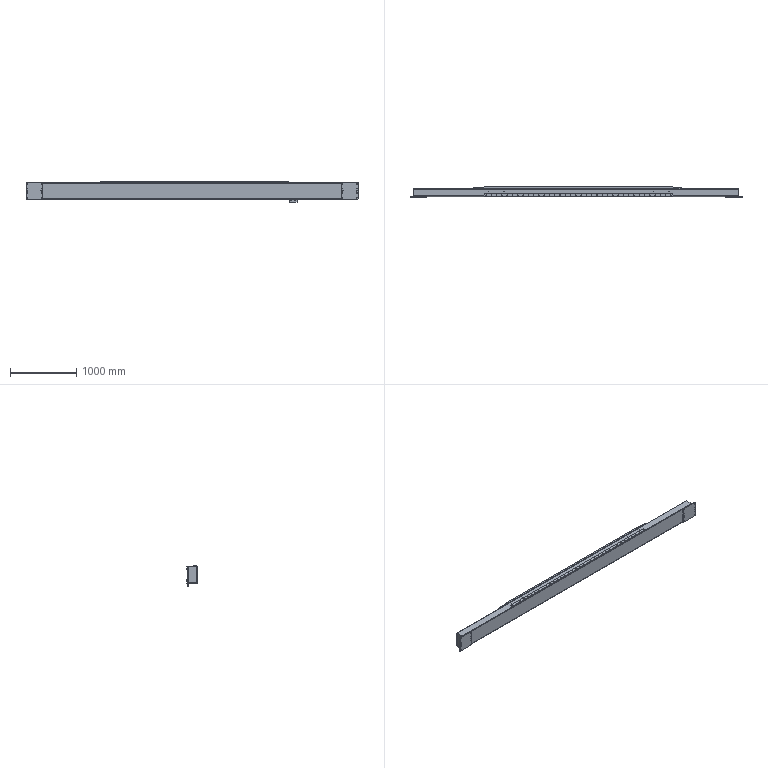Part | SolidWorks | features ICE 11, HoleWzd 10, Chamfer 1, MirrorSolid 1, WeldMemberFeat 1, WeldmentFeature 1 | 10 solids | 698 faces | box 5030 x 162 x 315 mm | volume 22440671 mm3 | cylinder 456 | cone 152 | plane 90 | commonest cylinder face diameters 6.8 x288 9 x48 8.5 x36 5 x24 15 x16 14 x12